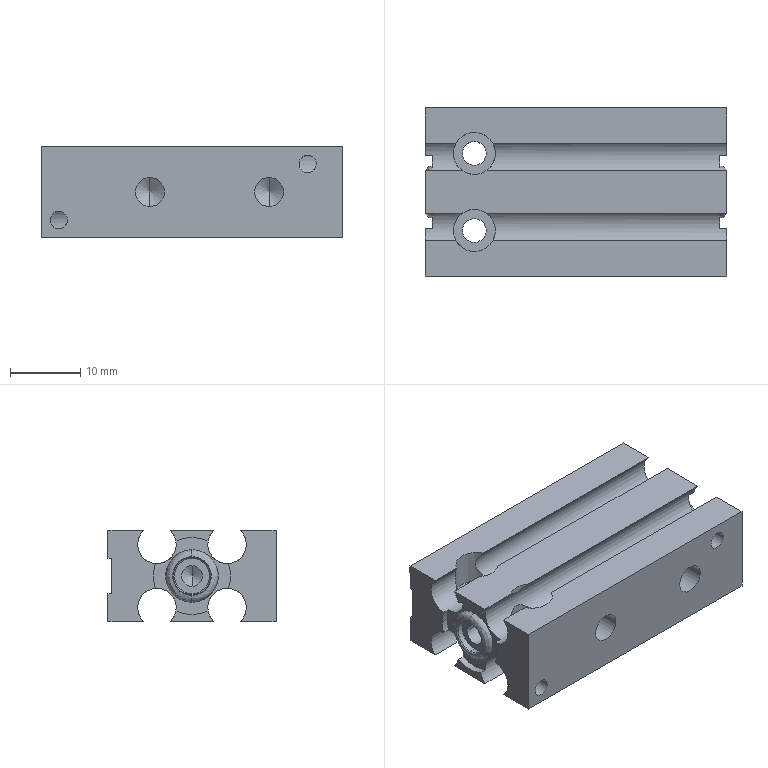Part | SolidWorks | features BaseBody 1 | 1 solid | 92 faces | box 43 x 24 x 13 mm | volume 9011 mm3 | cylinder 48 | plane 30 | cone 10 | spline 4 | commonest cylinder face diameters 6 x12 11 x10 5.5 x8 2.459 x4 3.4 x4 4.134 x4